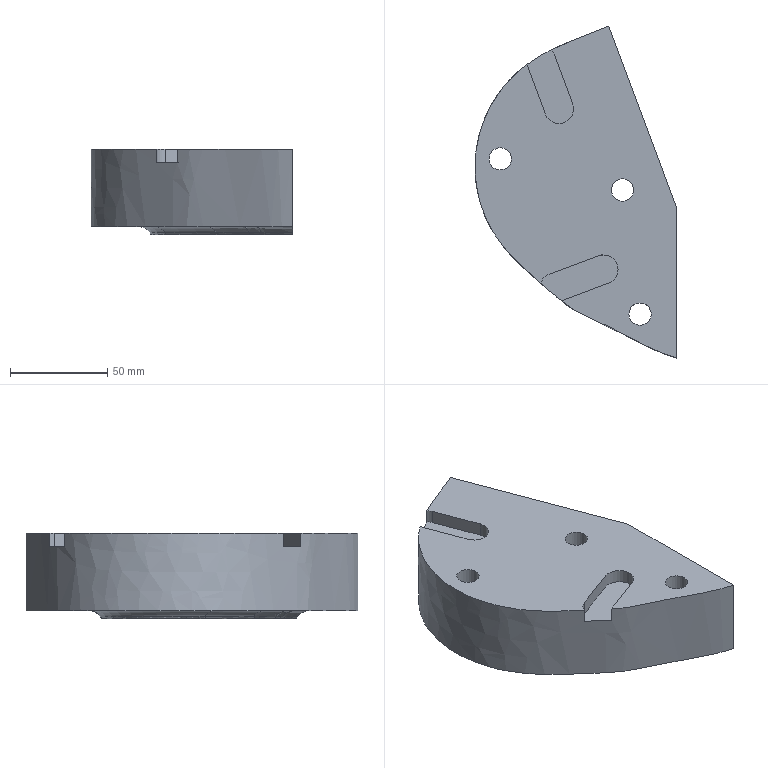Part | NX | features 8 2 | 1 solid | 52 faces | box 104.054 x 170.949 x 44.079 mm | volume 450697 mm3 | plane 14 | spline 13 | cylinder 13 | torus 10 | cone 2 | commonest cylinder face diameters 15 x5 11.5 x3 18 x3 8.5 x2